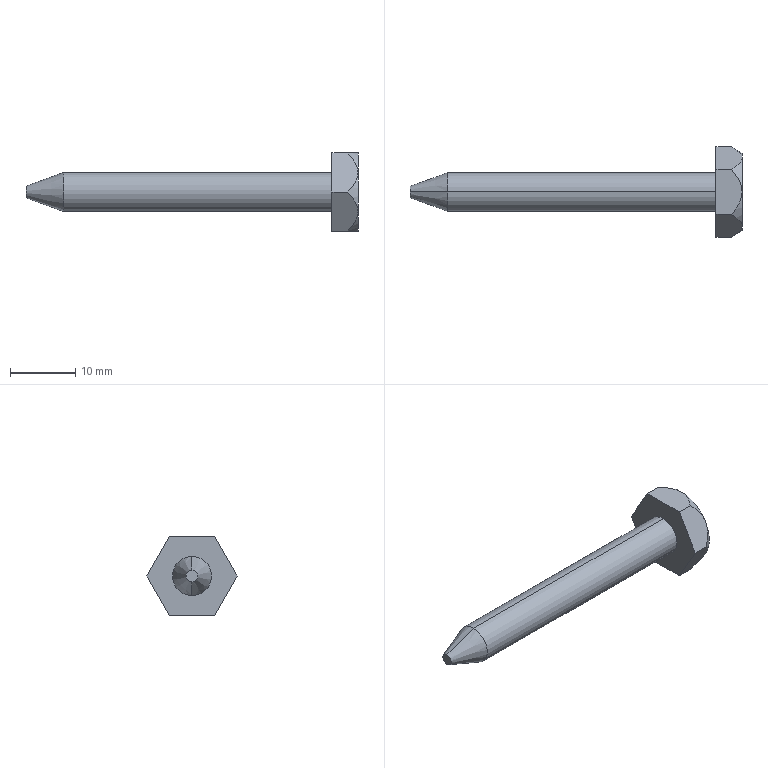Part | SolidWorks | features Extrusion 1, ICE 1, Revolution 1 | 1 solid | 19 faces | box 51 x 13.856 x 12 mm | volume 1735 mm3 | plane 9 | cone 8 | cylinder 2 | commonest cylinder face diameters 6 x2
STEP:
#1=CARTESIAN_POINT('',(-47.,0.,0.9));
#2=VERTEX_POINT('',#1);
#3=CARTESIAN_POINT('',(-47.,0.,-0.9));
#4=VERTEX_POINT('',#3);
#5=CARTESIAN_POINT('',(-47.,0.,0.));
#6=DIRECTION('',(-1.,0.,0.));
#7=DIRECTION('',(0.,0.,1.));
#8=AXIS2_PLACEMENT_3D('',#5,#6,#7);
#9=CIRCLE('',#8,0.9);
#10=EDGE_CURVE('',#2,#4,#9,.T.);
#11=ORIENTED_EDGE('',*,*,#10,.F.);
#12=CARTESIAN_POINT('',(-41.23,0.,3.));
#13=VERTEX_POINT('',#12);
#14=CARTESIAN_POINT('',(-41.23,0.,3.));
#15=DIRECTION('',(0.9397,0.,0.342));
#16=VECTOR('',#15,1000.);
#17=LINE('',#14,#16);
#18=EDGE_CURVE('',#2,#13,#17,.T.);
#19=ORIENTED_EDGE('',*,*,#18,.T.);
#20=CARTESIAN_POINT('',(-41.23,0.,-3.));
#21=VERTEX_POINT('',#20);
#22=CARTESIAN_POINT('',(-41.23,0.,0.));
#23=DIRECTION('',(-1.,0.,0.));
#24=DIRECTION('',(0.,0.,1.));
#25=AXIS2_PLACEMENT_3D('',#22,#23,#24);
#26=CIRCLE('',#25,3.);
#27=EDGE_CURVE('',#13,#21,#26,.T.);
#28=ORIENTED_EDGE('',*,*,#27,.T.);
#29=CARTESIAN_POINT('',(-41.23,0.,-3.));
#30=DIRECTION('',(0.9397,0.,-0.342));
#31=VECTOR('',#30,1000.);
#32=LINE('',#29,#31);
#33=EDGE_CURVE('',#4,#21,#32,.T.);
#34=ORIENTED_EDGE('',*,*,#33,.F.);
#35=EDGE_LOOP('',(#11,#19,#28,#34));
#36=FACE_OUTER_BOUND('',#35,.T.);
#37=CARTESIAN_POINT('',(-41.23,0.,0.));
#38=DIRECTION('',(1.,0.,0.));
#39=DIRECTION('',(0.,0.,-1.));
#40=AXIS2_PLACEMENT_3D('',#37,#38,#39);
#41=CONICAL_SURFACE('',#40,3.,0.3491);
#42=ADVANCED_FACE('',(#36),#41,.T.);
#43=CARTESIAN_POINT('',(0.,0.,3.));
#44=VERTEX_POINT('',#43);
#45=CARTESIAN_POINT('',(0.,0.,-3.));
#46=VERTEX_POINT('',#45);
#47=CARTESIAN_POINT('',(0.,0.,0.));
#48=DIRECTION('',(-1.,0.,0.));
#49=DIRECTION('',(0.,0.,1.));
#50=AXIS2_PLACEMENT_3D('',#47,#48,#49);
#51=CIRCLE('',#50,3.);
#52=EDGE_CURVE('',#44,#46,#51,.T.);
#53=ORIENTED_EDGE('',*,*,#52,.T.);
#54=CARTESIAN_POINT('',(-32.199,0.,-3.));
#55=DIRECTION('',(-1.,0.,0.));
#56=VECTOR('',#55,1000.);
#57=LINE('',#54,#56);
#58=EDGE_CURVE('',#46,#21,#57,.T.);
#59=ORIENTED_EDGE('',*,*,#58,.T.);
#60=ORIENTED_EDGE('',*,*,#27,.F.);
#61=CARTESIAN_POINT('',(-32.199,0.,3.));
#62=DIRECTION('',(-1.,0.,0.));
#63=VECTOR('',#62,1000.);
#64=LINE('',#61,#63);
#65=EDGE_CURVE('',#44,#13,#64,.T.);
#66=ORIENTED_EDGE('',*,*,#65,.F.);
#67=EDGE_LOOP('',(#53,#59,#60,#66));
#68=FACE_OUTER_BOUND('',#67,.T.);
#69=CARTESIAN_POINT('',(-32.199,0.,0.));
#70=DIRECTION('',(-1.,0.,0.));
#71=DIRECTION('',(0.,0.,1.));
#72=AXIS2_PLACEMENT_3D('',#69,#70,#71);
#73=CYLINDRICAL_SURFACE('',#72,3.);
#74=ADVANCED_FACE('',(#68),#73,.T.);
#75=CARTESIAN_POINT('',(2.392,-3.464,6.));
#76=VERTEX_POINT('',#75);
#77=CARTESIAN_POINT('',(4.,-5.196,3.));
#78=VERTEX_POINT('',#77);
#79=CARTESIAN_POINT('',(2.392,-3.464,6.));
#80=CARTESIAN_POINT('',(2.819,-3.711,5.573));
#81=CARTESIAN_POINT('',(3.206,-3.97,5.124));
#82=CARTESIAN_POINT('',(3.654,-4.403,4.374));
#83=CARTESIAN_POINT('',(3.78,-4.556,4.109));
#84=CARTESIAN_POINT('',(3.909,-4.791,3.702));
#85=CARTESIAN_POINT('',(3.943,-4.87,3.564));
#86=CARTESIAN_POINT('',(3.988,-5.032,3.284));
#87=CARTESIAN_POINT('',(4.,-5.115,3.141));
#88=CARTESIAN_POINT('',(4.,-5.196,3.));
#89=B_SPLINE_CURVE_WITH_KNOTS('',3,(#79,#80,#81,#82,#83,#84,#85,#86,#87,#88),.UNSPECIFIED.,.F.,.F.,(4,2,2,2,4),(0.000000303,0.001939,0.002909,0.003393,0.003878),.UNSPECIFIED.);
#90=EDGE_CURVE('',#76,#78,#89,.T.);
#91=ORIENTED_EDGE('',*,*,#90,.F.);
#92=CARTESIAN_POINT('',(0.,-3.464,6.));
#93=VERTEX_POINT('',#92);
#94=CARTESIAN_POINT('',(4.,-3.464,6.));
#95=DIRECTION('',(-1.,0.,0.));
#96=VECTOR('',#95,1000.);
#97=LINE('',#94,#96);
#98=EDGE_CURVE('',#76,#93,#97,.T.);
#99=ORIENTED_EDGE('',*,*,#98,.T.);
#100=CARTESIAN_POINT('',(0.,-6.928,0.));
#101=VERTEX_POINT('',#100);
#102=CARTESIAN_POINT('',(0.,-3.464,6.));
#103=DIRECTION('',(0.,-0.5,-0.866));
#104=VECTOR('',#103,1000.);
#105=LINE('',#102,#104);
#106=EDGE_CURVE('',#93,#101,#105,.T.);
#107=ORIENTED_EDGE('',*,*,#106,.T.);
#108=CARTESIAN_POINT('',(2.392,-6.928,0.));
#109=VERTEX_POINT('',#108);
#110=CARTESIAN_POINT('',(4.,-6.928,0.));
#111=DIRECTION('',(-1.,0.,0.));
#112=VECTOR('',#111,1000.);
#113=LINE('',#110,#112);
#114=EDGE_CURVE('',#109,#101,#113,.T.);
#115=ORIENTED_EDGE('',*,*,#114,.F.);
#116=CARTESIAN_POINT('',(4.,-5.196,3.));
#117=CARTESIAN_POINT('',(4.,-5.359,2.718));
#118=CARTESIAN_POINT('',(3.954,-5.519,2.441));
#119=CARTESIAN_POINT('',(3.781,-5.835,1.893));
#120=CARTESIAN_POINT('',(3.657,-5.985,1.633));
#121=CARTESIAN_POINT('',(3.361,-6.273,1.135));
#122=CARTESIAN_POINT('',(3.187,-6.412,0.8948));
#123=CARTESIAN_POINT('',(2.81,-6.678,0.4342));
#124=CARTESIAN_POINT('',(2.606,-6.805,0.2137));
#125=CARTESIAN_POINT('',(2.392,-6.928,0.));
#126=B_SPLINE_CURVE_WITH_KNOTS('',3,(#116,#117,#118,#119,#120,#121,#122,#123,#124,#125),.UNSPECIFIED.,.F.,.F.,(4,2,2,2,4),(0.003878,0.004846,0.005814,0.006782,0.00775),.UNSPECIFIED.);
#127=EDGE_CURVE('',#78,#109,#126,.T.);
#128=ORIENTED_EDGE('',*,*,#127,.F.);
#129=EDGE_LOOP('',(#91,#99,#107,#115,#128));
#130=FACE_OUTER_BOUND('',#129,.T.);
#131=CARTESIAN_POINT('',(4.,-3.464,6.));
#132=DIRECTION('',(0.,0.866,-0.5));
#133=DIRECTION('',(0.,0.5,0.866));
#134=AXIS2_PLACEMENT_3D('',#131,#132,#133);
#135=PLANE('',#134);
#136=ADVANCED_FACE('',(#130),#135,.F.);
#137=CARTESIAN_POINT('',(4.,-5.196,-3.));
#138=VERTEX_POINT('',#137);
#139=CARTESIAN_POINT('',(2.392,-6.928,0.));
#140=CARTESIAN_POINT('',(2.819,-6.682,-0.4268));
#141=CARTESIAN_POINT('',(3.206,-6.422,-0.8763));
#142=CARTESIAN_POINT('',(3.654,-5.989,-1.626));
#143=CARTESIAN_POINT('',(3.78,-5.836,-1.891));
#144=CARTESIAN_POINT('',(3.909,-5.601,-2.298));
#145=CARTESIAN_POINT('',(3.943,-5.522,-2.436));
#146=CARTESIAN_POINT('',(3.988,-5.36,-2.716));
#147=CARTESIAN_POINT('',(4.,-5.278,-2.859));
#148=CARTESIAN_POINT('',(4.,-5.196,-3.));
#149=B_SPLINE_CURVE_WITH_KNOTS('',3,(#139,#140,#141,#142,#143,#144,#145,#146,#147,#148),.UNSPECIFIED.,.F.,.F.,(4,2,2,2,4),(0.000000303,0.001939,0.002909,0.003393,0.003878),.UNSPECIFIED.);
#150=EDGE_CURVE('',#109,#138,#149,.T.);
#151=ORIENTED_EDGE('',*,*,#150,.F.);
#152=ORIENTED_EDGE('',*,*,#114,.T.);
#153=CARTESIAN_POINT('',(0.,-3.464,-6.));
#154=VERTEX_POINT('',#153);
#155=CARTESIAN_POINT('',(0.,-6.928,0.));
#156=DIRECTION('',(0.,0.5,-0.866));
#157=VECTOR('',#156,1000.);
#158=LINE('',#155,#157);
#159=EDGE_CURVE('',#101,#154,#158,.T.);
#160=ORIENTED_EDGE('',*,*,#159,.T.);
#161=CARTESIAN_POINT('',(2.392,-3.464,-6.));
#162=VERTEX_POINT('',#161);
#163=CARTESIAN_POINT('',(4.,-3.464,-6.));
#164=DIRECTION('',(-1.,0.,0.));
#165=VECTOR('',#164,1000.);
#166=LINE('',#163,#165);
#167=EDGE_CURVE('',#162,#154,#166,.T.);
#168=ORIENTED_EDGE('',*,*,#167,.F.);
#169=CARTESIAN_POINT('',(4.,-5.196,-3.));
#170=CARTESIAN_POINT('',(4.,-5.034,-3.282));
#171=CARTESIAN_POINT('',(3.954,-4.873,-3.559));
#172=CARTESIAN_POINT('',(3.781,-4.557,-4.107));
#173=CARTESIAN_POINT('',(3.657,-4.407,-4.367));
#174=CARTESIAN_POINT('',(3.361,-4.119,-4.865));
#175=CARTESIAN_POINT('',(3.187,-3.981,-5.105));
#176=CARTESIAN_POINT('',(2.81,-3.715,-5.566));
#177=CARTESIAN_POINT('',(2.606,-3.587,-5.786));
#178=CARTESIAN_POINT('',(2.392,-3.464,-6.));
#179=B_SPLINE_CURVE_WITH_KNOTS('',3,(#169,#170,#171,#172,#173,#174,#175,#176,#177,#178),.UNSPECIFIED.,.F.,.F.,(4,2,2,2,4),(0.003878,0.004846,0.005814,0.006782,0.00775),.UNSPECIFIED.);
#180=EDGE_CURVE('',#138,#162,#179,.T.);
#181=ORIENTED_EDGE('',*,*,#180,.F.);
#182=EDGE_LOOP('',(#151,#152,#160,#168,#181));
#183=FACE_OUTER_BOUND('',#182,.T.);
#184=CARTESIAN_POINT('',(4.,-6.928,0.));
#185=DIRECTION('',(0.,0.866,0.5));
#186=DIRECTION('',(0.,-0.5,0.866));
#187=AXIS2_PLACEMENT_3D('',#184,#185,#186);
#188=PLANE('',#187);
#189=ADVANCED_FACE('',(#183),#188,.F.);
#190=CARTESIAN_POINT('',(4.,0.,-6.));
#191=VERTEX_POINT('',#190);
#192=CARTESIAN_POINT('',(2.392,-3.464,-6.));
#193=CARTESIAN_POINT('',(2.604,-3.219,-6.));
#194=CARTESIAN_POINT('',(2.807,-2.967,-6.));
#195=CARTESIAN_POINT('',(3.183,-2.437,-6.));
#196=CARTESIAN_POINT('',(3.358,-2.158,-6.));
#197=CARTESIAN_POINT('',(3.657,-1.579,-6.));
#198=CARTESIAN_POINT('',(3.781,-1.278,-6.));
#199=CARTESIAN_POINT('',(3.954,-0.6439,-6.));
#200=CARTESIAN_POINT('',(4.,-0.3237,-6.));
#201=CARTESIAN_POINT('',(4.,0.,-6.));
#202=B_SPLINE_CURVE_WITH_KNOTS('',3,(#192,#193,#194,#195,#196,#197,#198,#199,#200,#201),.UNSPECIFIED.,.F.,.F.,(4,2,2,2,4),(0.01314,0.01411,0.01509,0.01606,0.01704),.UNSPECIFIED.);
#203=EDGE_CURVE('',#162,#191,#202,.T.);
#204=ORIENTED_EDGE('',*,*,#203,.F.);
#205=ORIENTED_EDGE('',*,*,#167,.T.);
#206=CARTESIAN_POINT('',(0.,3.464,-6.));
#207=VERTEX_POINT('',#206);
#208=CARTESIAN_POINT('',(0.,-3.464,-6.));
#209=DIRECTION('',(0.,1.,0.));
#210=VECTOR('',#209,1000.);
#211=LINE('',#208,#210);
#212=EDGE_CURVE('',#154,#207,#211,.T.);
#213=ORIENTED_EDGE('',*,*,#212,.T.);
#214=CARTESIAN_POINT('',(2.392,3.464,-6.));
#215=VERTEX_POINT('',#214);
#216=CARTESIAN_POINT('',(4.,3.464,-6.));
#217=DIRECTION('',(-1.,0.,0.));
#218=VECTOR('',#217,1000.);
#219=LINE('',#216,#218);
#220=EDGE_CURVE('',#215,#207,#219,.T.);
#221=ORIENTED_EDGE('',*,*,#220,.F.);
#222=CARTESIAN_POINT('',(4.,0.,-6.));
#223=CARTESIAN_POINT('',(4.,0.3232,-6.));
#224=CARTESIAN_POINT('',(3.952,0.6524,-6.));
#225=CARTESIAN_POINT('',(3.78,1.279,-6.));
#226=CARTESIAN_POINT('',(3.655,1.584,-6.));
#227=CARTESIAN_POINT('',(3.207,2.452,-6.));
#228=CARTESIAN_POINT('',(2.819,2.972,-6.));
#229=CARTESIAN_POINT('',(2.392,3.464,-6.));
#230=B_SPLINE_CURVE_WITH_KNOTS('',3,(#222,#223,#224,#225,#226,#227,#228,#229),.UNSPECIFIED.,.F.,.F.,(4,2,2,4),(0.01704,0.01801,0.01898,0.02093),.UNSPECIFIED.);
#231=EDGE_CURVE('',#191,#215,#230,.T.);
#232=ORIENTED_EDGE('',*,*,#231,.F.);
#233=EDGE_LOOP('',(#204,#205,#213,#221,#232));
#234=FACE_OUTER_BOUND('',#233,.T.);
#235=CARTESIAN_POINT('',(4.,-3.464,-6.));
#236=DIRECTION('',(0.,0.,1.));
#237=DIRECTION('',(0.,-1.,0.));
#238=AXIS2_PLACEMENT_3D('',#235,#236,#237);
#239=PLANE('',#238);
#240=ADVANCED_FACE('',(#234),#239,.F.);
#241=CARTESIAN_POINT('',(4.,5.196,-3.));
#242=VERTEX_POINT('',#241);
#243=CARTESIAN_POINT('',(2.392,3.464,-6.));
#244=CARTESIAN_POINT('',(2.819,3.711,-5.573));
#245=CARTESIAN_POINT('',(3.206,3.97,-5.124));
#246=CARTESIAN_POINT('',(3.654,4.403,-4.374));
#247=CARTESIAN_POINT('',(3.78,4.556,-4.109));
#248=CARTESIAN_POINT('',(3.909,4.791,-3.702));
#249=CARTESIAN_POINT('',(3.943,4.87,-3.564));
#250=CARTESIAN_POINT('',(3.988,5.032,-3.284));
#251=CARTESIAN_POINT('',(4.,5.115,-3.141));
#252=CARTESIAN_POINT('',(4.,5.196,-3.));
#253=B_SPLINE_CURVE_WITH_KNOTS('',3,(#243,#244,#245,#246,#247,#248,#249,#250,#251,#252),.UNSPECIFIED.,.F.,.F.,(4,2,2,2,4),(0.000000303,0.001939,0.002909,0.003393,0.003878),.UNSPECIFIED.);
#254=EDGE_CURVE('',#215,#242,#253,.T.);
#255=ORIENTED_EDGE('',*,*,#254,.F.);
#256=ORIENTED_EDGE('',*,*,#220,.T.);
#257=CARTESIAN_POINT('',(0.,6.928,0.));
#258=VERTEX_POINT('',#257);
#259=CARTESIAN_POINT('',(0.,3.464,-6.));
#260=DIRECTION('',(0.,0.5,0.866));
#261=VECTOR('',#260,1000.);
#262=LINE('',#259,#261);
#263=EDGE_CURVE('',#207,#258,#262,.T.);
#264=ORIENTED_EDGE('',*,*,#263,.T.);
#265=CARTESIAN_POINT('',(2.392,6.928,0.));
#266=VERTEX_POINT('',#265);
#267=CARTESIAN_POINT('',(4.,6.928,0.));
#268=DIRECTION('',(-1.,0.,0.));
#269=VECTOR('',#268,1000.);
#270=LINE('',#267,#269);
#271=EDGE_CURVE('',#266,#258,#270,.T.);
#272=ORIENTED_EDGE('',*,*,#271,.F.);
#273=CARTESIAN_POINT('',(4.,5.196,-3.));
#274=CARTESIAN_POINT('',(4.,5.359,-2.718));
#275=CARTESIAN_POINT('',(3.954,5.519,-2.441));
#276=CARTESIAN_POINT('',(3.781,5.835,-1.893));
#277=CARTESIAN_POINT('',(3.657,5.985,-1.633));
#278=CARTESIAN_POINT('',(3.361,6.273,-1.135));
#279=CARTESIAN_POINT('',(3.187,6.412,-0.8948));
#280=CARTESIAN_POINT('',(2.81,6.678,-0.4342));
#281=CARTESIAN_POINT('',(2.606,6.805,-0.2137));
#282=CARTESIAN_POINT('',(2.392,6.928,0.));
#283=B_SPLINE_CURVE_WITH_KNOTS('',3,(#273,#274,#275,#276,#277,#278,#279,#280,#281,#282),.UNSPECIFIED.,.F.,.F.,(4,2,2,2,4),(0.003878,0.004846,0.005814,0.006782,0.00775),.UNSPECIFIED.);
#284=EDGE_CURVE('',#242,#266,#283,.T.);
#285=ORIENTED_EDGE('',*,*,#284,.F.);
#286=EDGE_LOOP('',(#255,#256,#264,#272,#285));
#287=FACE_OUTER_BOUND('',#286,.T.);
#288=CARTESIAN_POINT('',(4.,3.464,-6.));
#289=DIRECTION('',(0.,-0.866,0.5));
#290=DIRECTION('',(0.,-0.5,-0.866));
#291=AXIS2_PLACEMENT_3D('',#288,#289,#290);
#292=PLANE('',#291);
#293=ADVANCED_FACE('',(#287),#292,.F.);
#294=CARTESIAN_POINT('',(4.,5.196,3.));
#295=VERTEX_POINT('',#294);
#296=CARTESIAN_POINT('',(2.392,6.928,0.));
#297=CARTESIAN_POINT('',(2.819,6.682,0.4268));
#298=CARTESIAN_POINT('',(3.206,6.422,0.8763));
#299=CARTESIAN_POINT('',(3.654,5.989,1.626));
#300=CARTESIAN_POINT('',(3.78,5.836,1.891));
#301=CARTESIAN_POINT('',(3.909,5.601,2.298));
#302=CARTESIAN_POINT('',(3.943,5.522,2.436));
#303=CARTESIAN_POINT('',(3.988,5.36,2.716));
#304=CARTESIAN_POINT('',(4.,5.278,2.859));
#305=CARTESIAN_POINT('',(4.,5.196,3.));
#306=B_SPLINE_CURVE_WITH_KNOTS('',3,(#296,#297,#298,#299,#300,#301,#302,#303,#304,#305),.UNSPECIFIED.,.F.,.F.,(4,2,2,2,4),(0.000000303,0.001939,0.002909,0.003393,0.003878),.UNSPECIFIED.);
#307=EDGE_CURVE('',#266,#295,#306,.T.);
#308=ORIENTED_EDGE('',*,*,#307,.F.);
#309=ORIENTED_EDGE('',*,*,#271,.T.);
#310=CARTESIAN_POINT('',(0.,3.464,6.));
#311=VERTEX_POINT('',#310);
#312=CARTESIAN_POINT('',(0.,6.928,0.));
#313=DIRECTION('',(0.,-0.5,0.866));
#314=VECTOR('',#313,1000.);
#315=LINE('',#312,#314);
#316=EDGE_CURVE('',#258,#311,#315,.T.);
#317=ORIENTED_EDGE('',*,*,#316,.T.);
#318=CARTESIAN_POINT('',(2.392,3.464,6.));
#319=VERTEX_POINT('',#318);
#320=CARTESIAN_POINT('',(4.,3.464,6.));
#321=DIRECTION('',(-1.,0.,0.));
#322=VECTOR('',#321,1000.);
#323=LINE('',#320,#322);
#324=EDGE_CURVE('',#319,#311,#323,.T.);
#325=ORIENTED_EDGE('',*,*,#324,.F.);
#326=CARTESIAN_POINT('',(4.,5.196,3.));
#327=CARTESIAN_POINT('',(4.,5.034,3.282));
#328=CARTESIAN_POINT('',(3.954,4.873,3.559));
#329=CARTESIAN_POINT('',(3.781,4.557,4.107));
#330=CARTESIAN_POINT('',(3.657,4.407,4.367));
#331=CARTESIAN_POINT('',(3.361,4.119,4.865));
#332=CARTESIAN_POINT('',(3.187,3.981,5.105));
#333=CARTESIAN_POINT('',(2.81,3.715,5.566));
#334=CARTESIAN_POINT('',(2.606,3.587,5.786));
#335=CARTESIAN_POINT('',(2.392,3.464,6.));
#336=B_SPLINE_CURVE_WITH_KNOTS('',3,(#326,#327,#328,#329,#330,#331,#332,#333,#334,#335),.UNSPECIFIED.,.F.,.F.,(4,2,2,2,4),(0.003878,0.004846,0.005814,0.006782,0.00775),.UNSPECIFIED.);
#337=EDGE_CURVE('',#295,#319,#336,.T.);
#338=ORIENTED_EDGE('',*,*,#337,.F.);
#339=EDGE_LOOP('',(#308,#309,#317,#325,#338));
#340=FACE_OUTER_BOUND('',#339,.T.);
#341=CARTESIAN_POINT('',(4.,6.928,0.));
#342=DIRECTION('',(0.,-0.866,-0.5));
#343=DIRECTION('',(0.,0.5,-0.866));
#344=AXIS2_PLACEMENT_3D('',#341,#342,#343);
#345=PLANE('',#344);
#346=ADVANCED_FACE('',(#340),#345,.F.);
#347=CARTESIAN_POINT('',(4.,0.,6.));
#348=VERTEX_POINT('',#347);
#349=CARTESIAN_POINT('',(2.392,3.464,6.));
#350=CARTESIAN_POINT('',(2.604,3.219,6.));
#351=CARTESIAN_POINT('',(2.807,2.967,6.));
#352=CARTESIAN_POINT('',(3.183,2.437,6.));
#353=CARTESIAN_POINT('',(3.358,2.158,6.));
#354=CARTESIAN_POINT('',(3.657,1.579,6.));
#355=CARTESIAN_POINT('',(3.781,1.278,6.));
#356=CARTESIAN_POINT('',(3.954,0.6439,6.));
#357=CARTESIAN_POINT('',(4.,0.3237,6.));
#358=CARTESIAN_POINT('',(4.,0.,6.));
#359=B_SPLINE_CURVE_WITH_KNOTS('',3,(#349,#350,#351,#352,#353,#354,#355,#356,#357,#358),.UNSPECIFIED.,.F.,.F.,(4,2,2,2,4),(0.01314,0.01411,0.01509,0.01606,0.01704),.UNSPECIFIED.);
#360=EDGE_CURVE('',#319,#348,#359,.T.);
#361=ORIENTED_EDGE('',*,*,#360,.F.);
#362=ORIENTED_EDGE('',*,*,#324,.T.);
#363=CARTESIAN_POINT('',(0.,3.464,6.));
#364=DIRECTION('',(0.,-1.,0.));
#365=VECTOR('',#364,1000.);
#366=LINE('',#363,#365);
#367=EDGE_CURVE('',#311,#93,#366,.T.);
#368=ORIENTED_EDGE('',*,*,#367,.T.);
#369=ORIENTED_EDGE('',*,*,#98,.F.);
#370=CARTESIAN_POINT('',(4.,0.,6.));
#371=CARTESIAN_POINT('',(4.,-0.3232,6.));
#372=CARTESIAN_POINT('',(3.952,-0.6524,6.));
#373=CARTESIAN_POINT('',(3.78,-1.279,6.));
#374=CARTESIAN_POINT('',(3.655,-1.584,6.));
#375=CARTESIAN_POINT('',(3.207,-2.452,6.));
#376=CARTESIAN_POINT('',(2.819,-2.972,6.));
#377=CARTESIAN_POINT('',(2.392,-3.464,6.));
#378=B_SPLINE_CURVE_WITH_KNOTS('',3,(#370,#371,#372,#373,#374,#375,#376,#377),.UNSPECIFIED.,.F.,.F.,(4,2,2,4),(0.01704,0.01801,0.01898,0.02093),.UNSPECIFIED.);
#379=EDGE_CURVE('',#348,#76,#378,.T.);
#380=ORIENTED_EDGE('',*,*,#379,.F.);
#381=EDGE_LOOP('',(#361,#362,#368,#369,#380));
#382=FACE_OUTER_BOUND('',#381,.T.);
#383=CARTESIAN_POINT('',(4.,3.464,6.));
#384=DIRECTION('',(0.,0.,-1.));
#385=DIRECTION('',(0.,1.,0.));
#386=AXIS2_PLACEMENT_3D('',#383,#384,#385);
#387=PLANE('',#386);
#388=ADVANCED_FACE('',(#382),#387,.F.);
#389=ORIENTED_EDGE('',*,*,#52,.F.);
#390=CARTESIAN_POINT('',(0.,0.,0.));
#391=DIRECTION('',(-1.,0.,0.));
#392=DIRECTION('',(0.,0.,1.));
#393=AXIS2_PLACEMENT_3D('',#390,#391,#392);
#394=CIRCLE('',#393,3.);
#395=EDGE_CURVE('',#46,#44,#394,.T.);
#396=ORIENTED_EDGE('',*,*,#395,.F.);
#397=EDGE_LOOP('',(#389,#396));
#398=FACE_BOUND('',#397,.T.);
#399=ORIENTED_EDGE('',*,*,#106,.F.);
#400=ORIENTED_EDGE('',*,*,#367,.F.);
#401=ORIENTED_EDGE('',*,*,#316,.F.);
#402=ORIENTED_EDGE('',*,*,#263,.F.);
#403=ORIENTED_EDGE('',*,*,#212,.F.);
#404=ORIENTED_EDGE('',*,*,#159,.F.);
#405=EDGE_LOOP('',(#399,#400,#401,#402,#403,#404));
#406=FACE_OUTER_BOUND('',#405,.T.);
#407=CARTESIAN_POINT('',(0.,0.,0.));
#408=DIRECTION('',(1.,0.,0.));
#409=DIRECTION('',(0.,0.,-1.));
#410=AXIS2_PLACEMENT_3D('',#407,#408,#409);
#411=PLANE('',#410);
#412=ADVANCED_FACE('',(#398,#406),#411,.F.);
#413=ORIENTED_EDGE('',*,*,#180,.T.);
#414=ORIENTED_EDGE('',*,*,#203,.T.);
#415=CARTESIAN_POINT('',(4.,0.,0.));
#416=DIRECTION('',(1.,0.,0.));
#417=DIRECTION('',(0.,0.,-1.));
#418=AXIS2_PLACEMENT_3D('',#415,#416,#417);
#419=CIRCLE('',#418,6.);
#420=EDGE_CURVE('',#138,#191,#419,.T.);
#421=ORIENTED_EDGE('',*,*,#420,.F.);
#422=EDGE_LOOP('',(#413,#414,#421));
#423=FACE_OUTER_BOUND('',#422,.T.);
#424=CARTESIAN_POINT('',(4.,0.,0.));
#425=DIRECTION('',(-1.,0.,0.));
#426=DIRECTION('',(0.,0.,-1.));
#427=AXIS2_PLACEMENT_3D('',#424,#425,#426);
#428=CONICAL_SURFACE('',#427,6.,0.5236);
#429=ADVANCED_FACE('',(#423),#428,.T.);
#430=ORIENTED_EDGE('',*,*,#127,.T.);
#431=ORIENTED_EDGE('',*,*,#150,.T.);
#432=CARTESIAN_POINT('',(4.,0.,0.));
#433=DIRECTION('',(1.,0.,0.));
#434=DIRECTION('',(0.,0.,-1.));
#435=AXIS2_PLACEMENT_3D('',#432,#433,#434);
#436=CIRCLE('',#435,6.);
#437=EDGE_CURVE('',#78,#138,#436,.T.);
#438=ORIENTED_EDGE('',*,*,#437,.F.);
#439=EDGE_LOOP('',(#430,#431,#438));
#440=FACE_OUTER_BOUND('',#439,.T.);
#441=CARTESIAN_POINT('',(4.,0.,0.));
#442=DIRECTION('',(-1.,0.,0.));
#443=DIRECTION('',(0.,0.,-1.));
#444=AXIS2_PLACEMENT_3D('',#441,#442,#443);
#445=CONICAL_SURFACE('',#444,6.,0.5236);
#446=ADVANCED_FACE('',(#440),#445,.T.);
#447=ORIENTED_EDGE('',*,*,#90,.T.);
#448=CARTESIAN_POINT('',(4.,0.,0.));
#449=DIRECTION('',(1.,0.,0.));
#450=DIRECTION('',(0.,0.,-1.));
#451=AXIS2_PLACEMENT_3D('',#448,#449,#450);
#452=CIRCLE('',#451,6.);
#453=EDGE_CURVE('',#348,#78,#452,.T.);
#454=ORIENTED_EDGE('',*,*,#453,.F.);
#455=ORIENTED_EDGE('',*,*,#379,.T.);
#456=EDGE_LOOP('',(#447,#454,#455));
#457=FACE_OUTER_BOUND('',#456,.T.);
#458=CARTESIAN_POINT('',(4.,0.,0.));
#459=DIRECTION('',(-1.,0.,0.));
#460=DIRECTION('',(0.,0.,-1.));
#461=AXIS2_PLACEMENT_3D('',#458,#459,#460);
#462=CONICAL_SURFACE('',#461,6.,0.5236);
#463=ADVANCED_FACE('',(#457),#462,.T.);
#464=ORIENTED_EDGE('',*,*,#337,.T.);
#465=ORIENTED_EDGE('',*,*,#360,.T.);
#466=CARTESIAN_POINT('',(4.,0.,0.));
#467=DIRECTION('',(1.,0.,0.));
#468=DIRECTION('',(0.,0.,-1.));
#469=AXIS2_PLACEMENT_3D('',#466,#467,#468);
#470=CIRCLE('',#469,6.);
#471=EDGE_CURVE('',#295,#348,#470,.T.);
#472=ORIENTED_EDGE('',*,*,#471,.F.);
#473=EDGE_LOOP('',(#464,#465,#472));
#474=FACE_OUTER_BOUND('',#473,.T.);
#475=CARTESIAN_POINT('',(4.,0.,0.));
#476=DIRECTION('',(-1.,0.,0.));
#477=DIRECTION('',(0.,0.,-1.));
#478=AXIS2_PLACEMENT_3D('',#475,#476,#477);
#479=CONICAL_SURFACE('',#478,6.,0.5236);
#480=ADVANCED_FACE('',(#474),#479,.T.);
#481=ORIENTED_EDGE('',*,*,#284,.T.);
#482=ORIENTED_EDGE('',*,*,#307,.T.);
#483=CARTESIAN_POINT('',(4.,0.,0.));
#484=DIRECTION('',(1.,0.,0.));
#485=DIRECTION('',(0.,0.,-1.));
#486=AXIS2_PLACEMENT_3D('',#483,#484,#485);
#487=CIRCLE('',#486,6.);
#488=EDGE_CURVE('',#242,#295,#487,.T.);
#489=ORIENTED_EDGE('',*,*,#488,.F.);
#490=EDGE_LOOP('',(#481,#482,#489));
#491=FACE_OUTER_BOUND('',#490,.T.);
#492=CARTESIAN_POINT('',(4.,0.,0.));
#493=DIRECTION('',(-1.,0.,0.));
#494=DIRECTION('',(0.,0.,-1.));
#495=AXIS2_PLACEMENT_3D('',#492,#493,#494);
#496=CONICAL_SURFACE('',#495,6.,0.5236);
#497=ADVANCED_FACE('',(#491),#496,.T.);
#498=ORIENTED_EDGE('',*,*,#231,.T.);
#499=ORIENTED_EDGE('',*,*,#254,.T.);
#500=CARTESIAN_POINT('',(4.,0.,0.));
#501=DIRECTION('',(1.,0.,0.));
#502=DIRECTION('',(0.,0.,-1.));
#503=AXIS2_PLACEMENT_3D('',#500,#501,#502);
#504=CIRCLE('',#503,6.);
#505=EDGE_CURVE('',#191,#242,#504,.T.);
#506=ORIENTED_EDGE('',*,*,#505,.F.);
#507=EDGE_LOOP('',(#498,#499,#506));
#508=FACE_OUTER_BOUND('',#507,.T.);
#509=CARTESIAN_POINT('',(4.,0.,0.));
#510=DIRECTION('',(-1.,0.,0.));
#511=DIRECTION('',(0.,0.,-1.));
#512=AXIS2_PLACEMENT_3D('',#509,#510,#511);
#513=CONICAL_SURFACE('',#512,6.,0.5236);
#514=ADVANCED_FACE('',(#508),#513,.T.);
#515=ORIENTED_EDGE('',*,*,#420,.T.);
#516=ORIENTED_EDGE('',*,*,#505,.T.);
#517=ORIENTED_EDGE('',*,*,#488,.T.);
#518=ORIENTED_EDGE('',*,*,#471,.T.);
#519=ORIENTED_EDGE('',*,*,#453,.T.);
#520=ORIENTED_EDGE('',*,*,#437,.T.);
#521=EDGE_LOOP('',(#515,#516,#517,#518,#519,#520));
#522=FACE_OUTER_BOUND('',#521,.T.);
#523=CARTESIAN_POINT('',(4.,0.,0.));
#524=DIRECTION('',(1.,0.,0.));
#525=DIRECTION('',(0.,0.,-1.));
#526=AXIS2_PLACEMENT_3D('',#523,#524,#525);
#527=PLANE('',#526);
#528=ADVANCED_FACE('',(#522),#527,.T.);
#529=ORIENTED_EDGE('',*,*,#58,.F.);
#530=ORIENTED_EDGE('',*,*,#395,.T.);
#531=ORIENTED_EDGE('',*,*,#65,.T.);
#532=CARTESIAN_POINT('',(-41.23,0.,0.));
#533=DIRECTION('',(-1.,0.,0.));
#534=DIRECTION('',(0.,0.,1.));
#535=AXIS2_PLACEMENT_3D('',#532,#533,#534);
#536=CIRCLE('',#535,3.);
#537=EDGE_CURVE('',#21,#13,#536,.T.);
#538=ORIENTED_EDGE('',*,*,#537,.F.);
#539=EDGE_LOOP('',(#529,#530,#531,#538));
#540=FACE_OUTER_BOUND('',#539,.T.);
#541=CARTESIAN_POINT('',(-32.199,0.,0.));
#542=DIRECTION('',(-1.,0.,0.));
#543=DIRECTION('',(0.,0.,1.));
#544=AXIS2_PLACEMENT_3D('',#541,#542,#543);
#545=CYLINDRICAL_SURFACE('',#544,3.);
#546=ADVANCED_FACE('',(#540),#545,.T.);
#547=ORIENTED_EDGE('',*,*,#18,.F.);
#548=CARTESIAN_POINT('',(-47.,0.,0.));
#549=DIRECTION('',(-1.,0.,0.));
#550=DIRECTION('',(0.,0.,1.));
#551=AXIS2_PLACEMENT_3D('',#548,#549,#550);
#552=CIRCLE('',#551,0.9);
#553=EDGE_CURVE('',#4,#2,#552,.T.);
#554=ORIENTED_EDGE('',*,*,#553,.F.);
#555=ORIENTED_EDGE('',*,*,#33,.T.);
#556=ORIENTED_EDGE('',*,*,#537,.T.);
#557=EDGE_LOOP('',(#547,#554,#555,#556));
#558=FACE_OUTER_BOUND('',#557,.T.);
#559=CARTESIAN_POINT('',(-41.23,0.,0.));
#560=DIRECTION('',(1.,0.,0.));
#561=DIRECTION('',(0.,0.,-1.));
#562=AXIS2_PLACEMENT_3D('',#559,#560,#561);
#563=CONICAL_SURFACE('',#562,3.,0.3491);
#564=ADVANCED_FACE('',(#558),#563,.T.);
#565=ORIENTED_EDGE('',*,*,#553,.T.);
#566=ORIENTED_EDGE('',*,*,#10,.T.);
#567=EDGE_LOOP('',(#565,#566));
#568=FACE_OUTER_BOUND('',#567,.T.);
#569=CARTESIAN_POINT('',(-47.,0.9,0.));
#570=DIRECTION('',(1.,0.,0.));
#571=DIRECTION('',(0.,0.,-1.));
#572=AXIS2_PLACEMENT_3D('',#569,#570,#571);
#573=PLANE('',#572);
#574=ADVANCED_FACE('',(#568),#573,.F.);
#575=CLOSED_SHELL('',(#42,#74,#136,#189,#240,#293,#346,#388,#412,#429,#446,#463,#480,#497,#514,#528,#546,#564,#574));
#576=MANIFOLD_SOLID_BREP('',#575);
#577=CARTESIAN_POINT('',(0.,0.,0.));
#578=DIRECTION('',(0.,0.,1.));
#579=DIRECTION('',(1.,0.,0.));
#580=AXIS2_PLACEMENT_3D('',#577,#578,#579);
#581=(LENGTH_UNIT()NAMED_UNIT(*)SI_UNIT(.MILLI.,.METRE.));
#582=UNCERTAINTY_MEASURE_WITH_UNIT(LENGTH_MEASURE(0.00001),#581,'','');
#583=(NAMED_UNIT(*)PLANE_ANGLE_UNIT()SI_UNIT($,.RADIAN.));
#584=(NAMED_UNIT(*)SI_UNIT($,.STERADIAN.)SOLID_ANGLE_UNIT());
#585=(GEOMETRIC_REPRESENTATION_CONTEXT(3)GLOBAL_UNCERTAINTY_ASSIGNED_CONTEXT((#582))GLOBAL_UNIT_ASSIGNED_CONTEXT((#581,#583,#584))REPRESENTATION_CONTEXT('',''));
#586=ADVANCED_BREP_SHAPE_REPRESENTATION('',(#576,#580),#585);